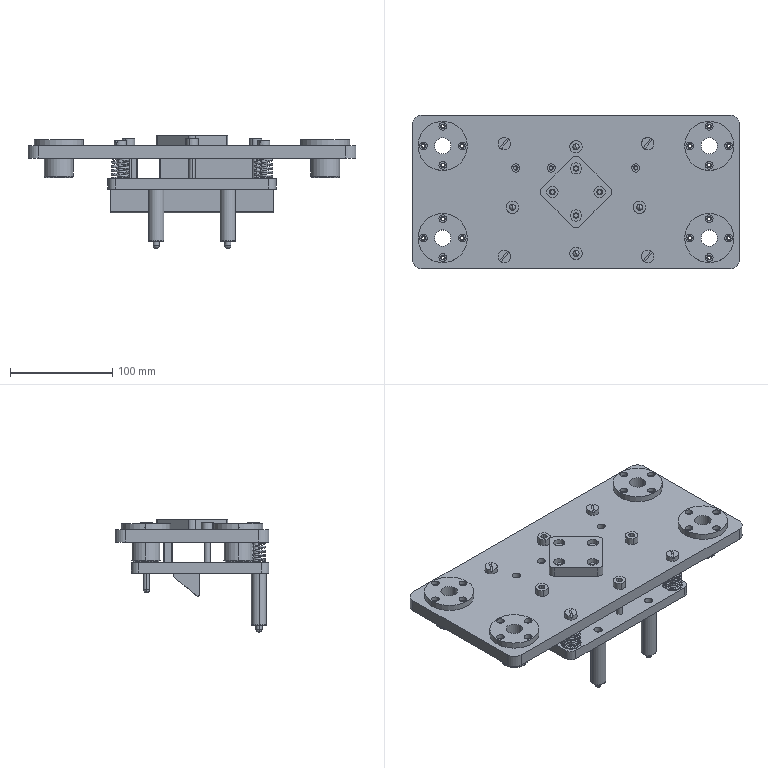Part | SolidWorks | 30 solids | 744 faces | box 320 x 150 x 110.25 mm | volume 967220 mm3 | cylinder 434 | plane 176 | torus 70 | spline 38 | sphere 16 | cone 10 | commonest cylinder face diameters 3.3 x44 6 x44 4.2 x36 4.5 x32 7.5 x32 12 x32